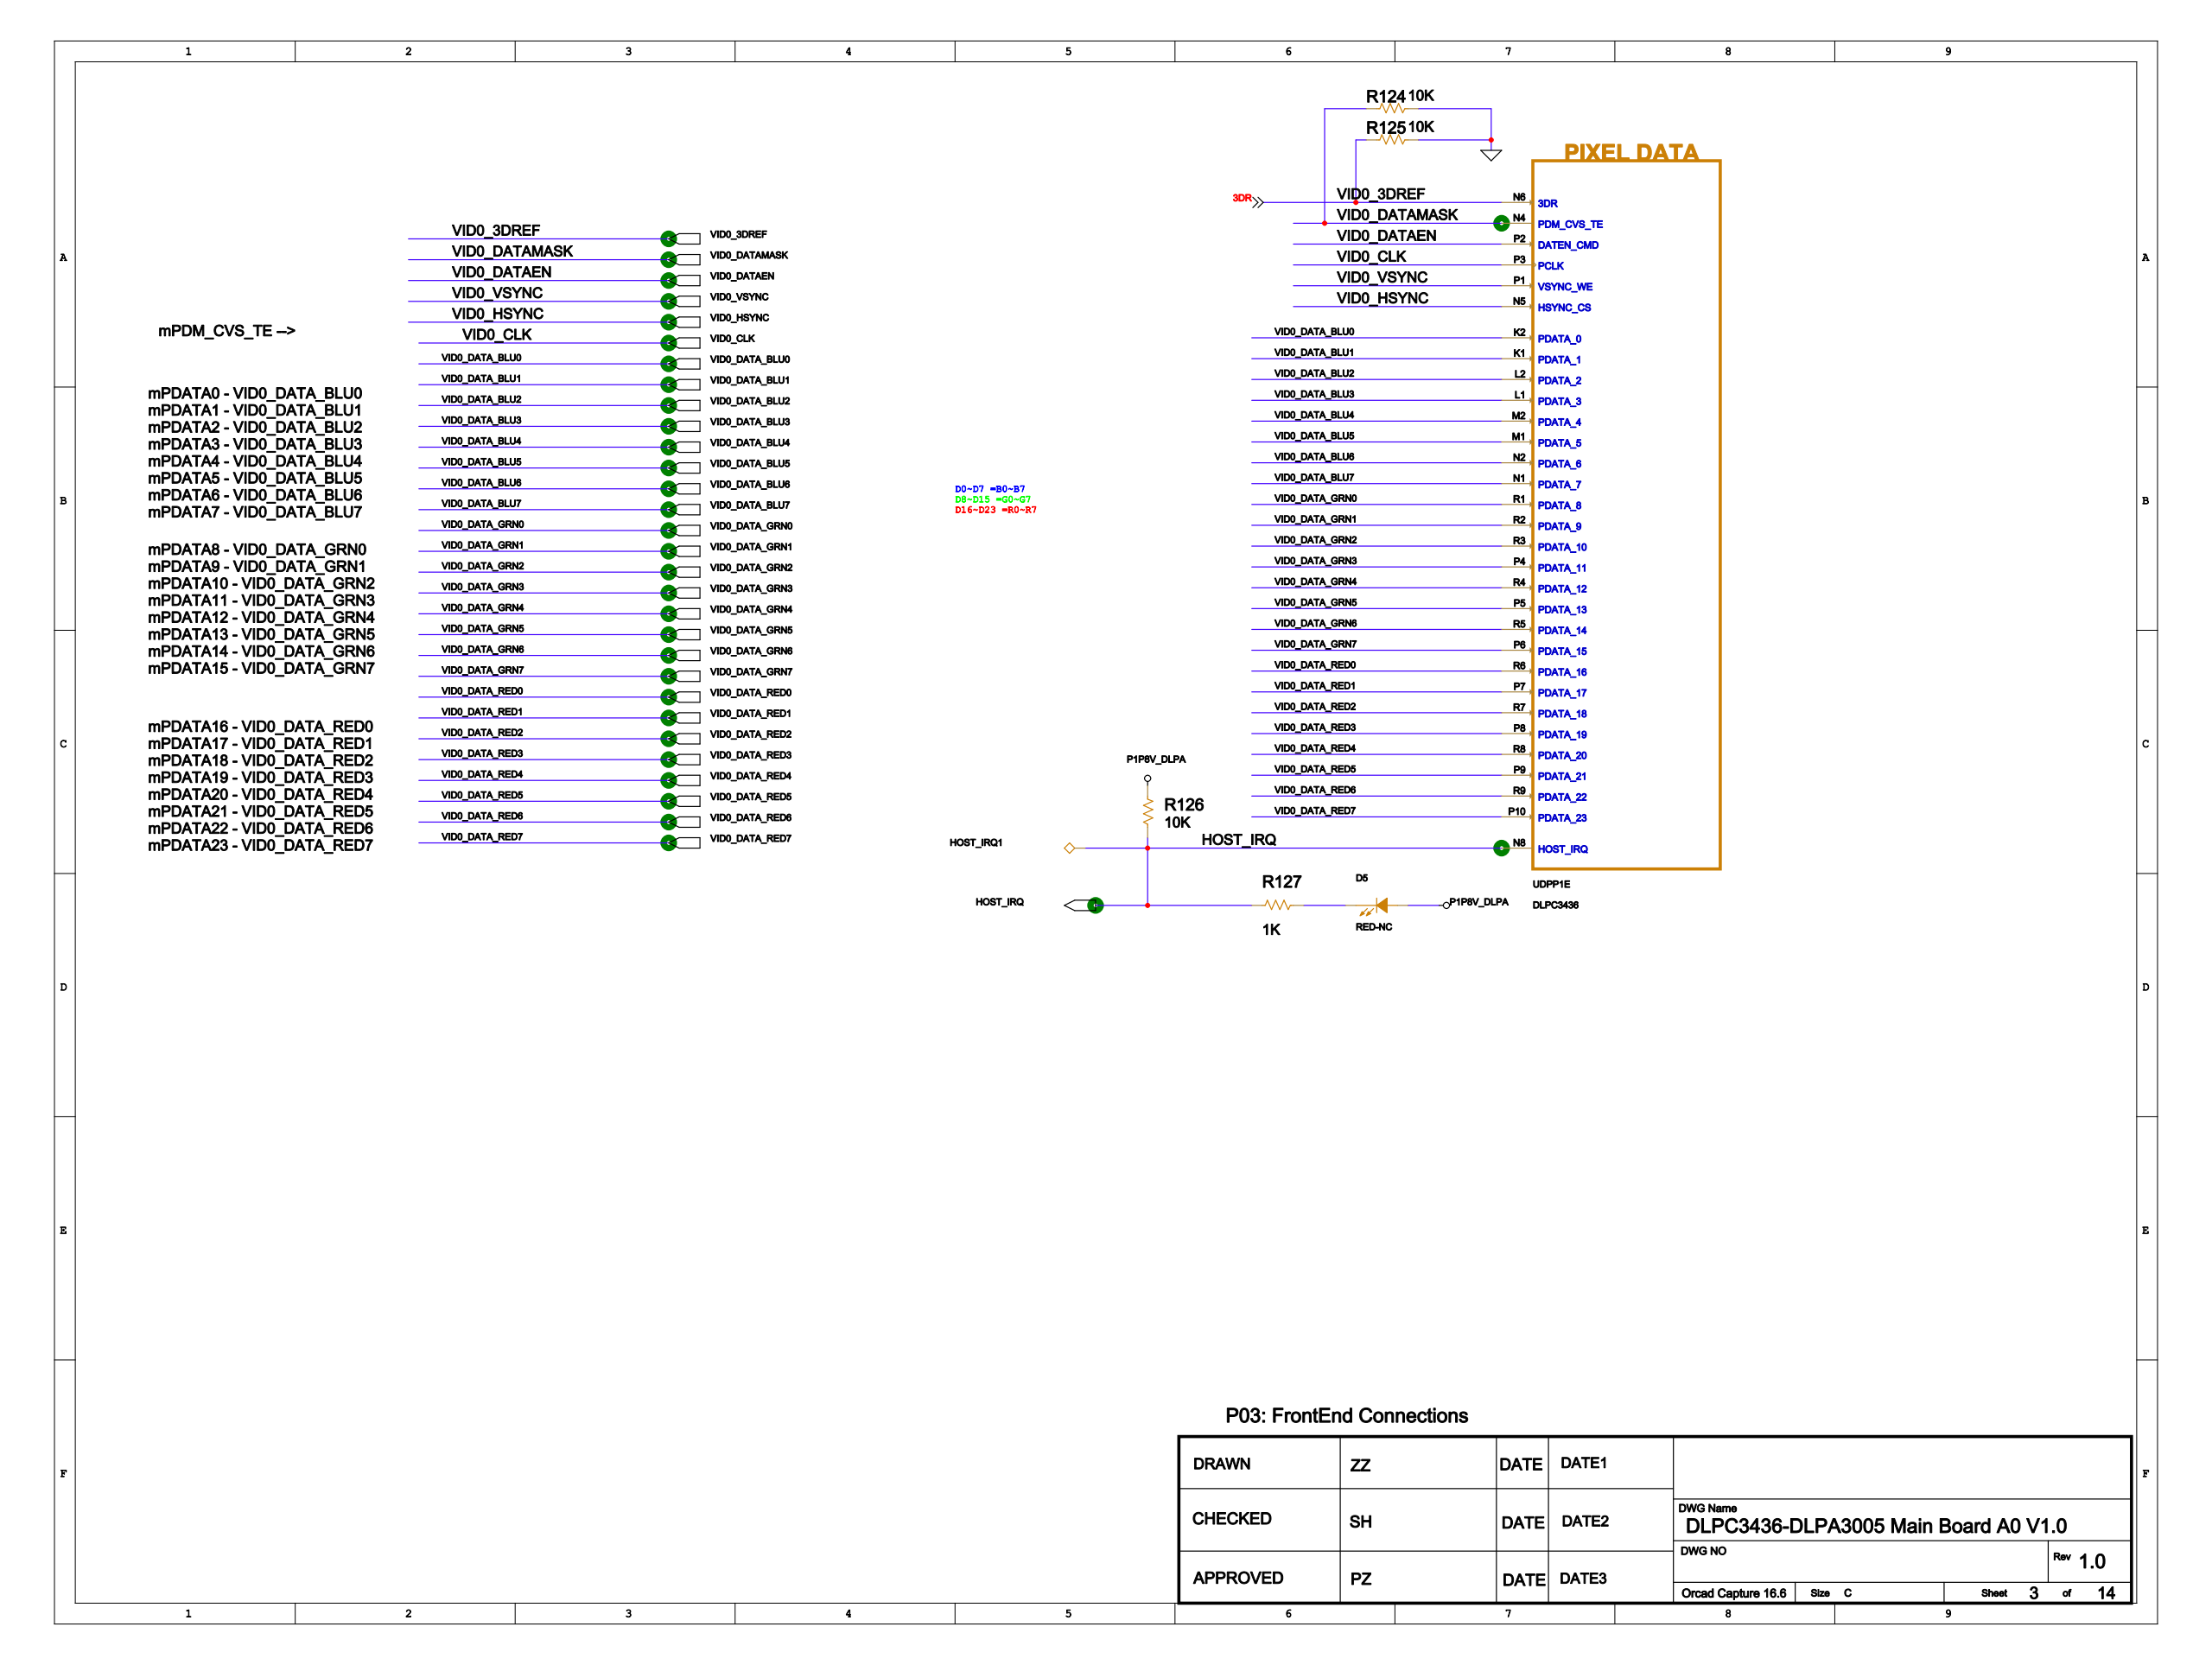Circuit board | Cadence Allegro | 1223 parts | 777 nets | one sheet of the schematic
Parts on this sheet (reference | value | footprint):
D5 | RED-NC | SMD-LED
HOST_IRQ1 | TP40 | TP06MM
R126 | 10K | R0201
R127 | 1K | R0201
UDPP1 | DLPC3436 | DLPC3436_176NFBGA
Nets of these parts (net: part-pin ...):
P1P8V_DLPA: D5-1 R126-1
N21910945: D5-2 R127-2
HOST_IRQ: HOST_IRQ1-1 R126-2 R127-1 UDPP1-N8
VID0_DATAMASK: UDPP1-N4
VID0_3DREF: UDPP1-N6
VID0_DATA_GRN6: UDPP1-R5
VID0_DATA_RED5: UDPP1-P9
VID0_DATA_GRN5: UDPP1-P5
VID0_DATA_GRN7: UDPP1-P6
VID0_CLK: UDPP1-P3
VID0_DATA_RED3: UDPP1-P8
VID0_DATA_RED4: UDPP1-R8
VID0_DATA_RED0: UDPP1-R6
VID0_DATA_RED2: UDPP1-R7
VID0_DATA_RED1: UDPP1-P7
VID0_DATA_RED6: UDPP1-R9
VID0_DATA_BLU6: UDPP1-N2
VID0_DATA_BLU5: UDPP1-M1
VID0_DATAEN: UDPP1-P2
VID0_DATA_RED7: UDPP1-P10
VID0_VSYNC: UDPP1-P1
VID0_HSYNC: UDPP1-N5
VID0_DATA_BLU0: UDPP1-K2
VID0_DATA_BLU2: UDPP1-L2
VID0_DATA_BLU1: UDPP1-K1
VID0_DATA_BLU7: UDPP1-N1
VID0_DATA_GRN3: UDPP1-P4
VID0_DATA_GRN2: UDPP1-R3
VID0_DATA_GRN1: UDPP1-R2
VID0_DATA_BLU4: UDPP1-M2
VID0_DATA_BLU3: UDPP1-L1
VID0_DATA_GRN0: UDPP1-R1
VID0_DATA_GRN4: UDPP1-R4